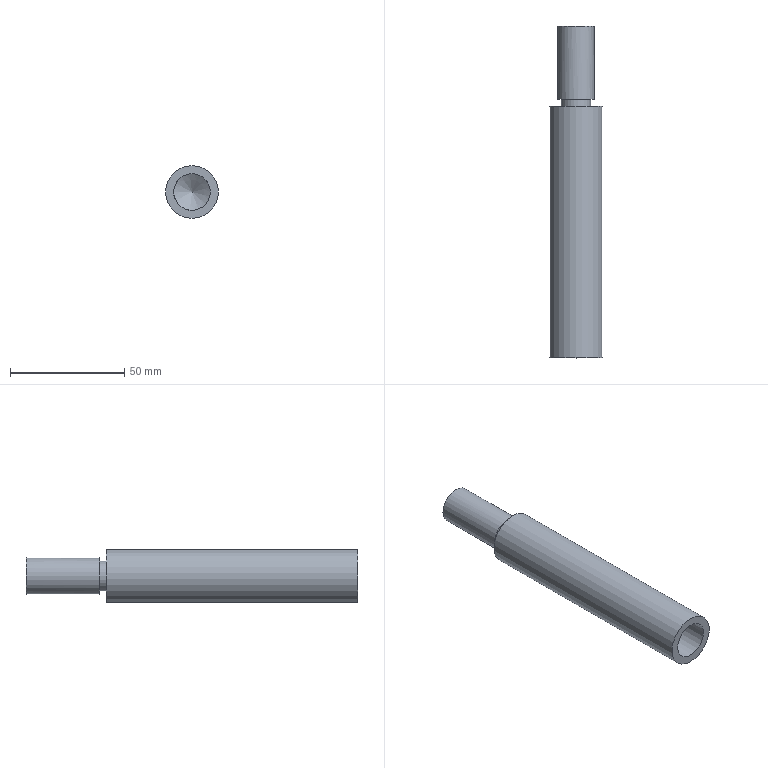Part | NX | features solid 2 | 1 solid | 9 faces | box 23 x 145 x 23 mm | volume 41355 mm3 | cylinder 4 | plane 4 | cone 1 | commonest cylinder face diameters 16 x2 13 x1 23 x1
STEP:
#1=CARTESIAN_POINT('',(288.,604.,-380.));
#2=VERTEX_POINT('',#1);
#3=CARTESIAN_POINT('',(280.,604.,-380.));
#4=DIRECTION('',(0.,-1.,0.));
#5=DIRECTION('',(1.,0.,0.));
#6=AXIS2_PLACEMENT_3D('',#3,#4,#5);
#7=CIRCLE('',#6,8.);
#8=EDGE_CURVE('',#2,#2,#7,.T.);
#9=ORIENTED_EDGE('',*,*,#8,.T.);
#10=EDGE_LOOP('',(#9));
#11=FACE_BOUND('',#10,.T.);
#12=CARTESIAN_POINT('',(280.,608.807,-380.));
#13=VERTEX_POINT('',#12);
#14=VERTEX_LOOP('',#13);
#15=FACE_BOUND('',#14,.T.);
#16=CARTESIAN_POINT('',(280.,604.,-380.));
#17=DIRECTION('',(0.,-1.,0.));
#18=DIRECTION('',(-1.,0.,0.));
#19=AXIS2_PLACEMENT_3D('',#16,#17,#18);
#20=CONICAL_SURFACE('',#19,8.,1.03);
#21=ADVANCED_FACE('',(#11,#15),#20,.F.);
#22=ORIENTED_EDGE('',*,*,#8,.F.);
#23=EDGE_LOOP('',(#22));
#24=FACE_BOUND('',#23,.T.);
#25=CARTESIAN_POINT('',(280.,550.,-372.));
#26=VERTEX_POINT('',#25);
#27=CARTESIAN_POINT('',(280.,550.,-380.));
#28=DIRECTION('',(0.,1.,0.));
#29=DIRECTION('',(0.,0.,1.));
#30=AXIS2_PLACEMENT_3D('',#27,#28,#29);
#31=CIRCLE('',#30,8.);
#32=EDGE_CURVE('',#26,#26,#31,.F.);
#33=ORIENTED_EDGE('',*,*,#32,.T.);
#34=EDGE_LOOP('',(#33));
#35=FACE_BOUND('',#34,.T.);
#36=CARTESIAN_POINT('',(280.,579.,-380.));
#37=DIRECTION('',(0.,1.,0.));
#38=DIRECTION('',(1.,0.,0.));
#39=AXIS2_PLACEMENT_3D('',#36,#37,#38);
#40=CYLINDRICAL_SURFACE('',#39,8.);
#41=ADVANCED_FACE('',(#24,#35),#40,.F.);
#42=CARTESIAN_POINT('',(280.,550.,-368.5));
#43=VERTEX_POINT('',#42);
#44=CARTESIAN_POINT('',(280.,550.,-380.));
#45=DIRECTION('',(0.,1.,0.));
#46=DIRECTION('',(0.,0.,1.));
#47=AXIS2_PLACEMENT_3D('',#44,#45,#46);
#48=CIRCLE('',#47,11.5);
#49=EDGE_CURVE('',#43,#43,#48,.T.);
#50=ORIENTED_EDGE('',*,*,#49,.F.);
#51=EDGE_LOOP('',(#50));
#52=FACE_BOUND('',#51,.T.);
#53=ORIENTED_EDGE('',*,*,#32,.F.);
#54=EDGE_LOOP('',(#53));
#55=FACE_BOUND('',#54,.T.);
#56=CARTESIAN_POINT('',(280.,550.,-380.));
#57=DIRECTION('',(0.,-1.,0.));
#58=DIRECTION('',(-1.,0.,0.));
#59=AXIS2_PLACEMENT_3D('',#56,#57,#58);
#60=PLANE('',#59);
#61=ADVANCED_FACE('',(#52,#55),#60,.T.);
#62=ORIENTED_EDGE('',*,*,#49,.T.);
#63=EDGE_LOOP('',(#62));
#64=FACE_BOUND('',#63,.T.);
#65=CARTESIAN_POINT('',(270.34,650.,-373.76));
#66=VERTEX_POINT('',#65);
#67=CARTESIAN_POINT('',(270.34,635.,-373.76));
#68=VERTEX_POINT('',#67);
#69=CARTESIAN_POINT('',(270.34,508.,-373.76));
#70=DIRECTION('',(0.,1.,0.));
#71=VECTOR('',#70,1000.);
#72=LINE('',#69,#71);
#73=EDGE_CURVE('',#66,#68,#72,.F.);
#74=ORIENTED_EDGE('',*,*,#73,.T.);
#75=ORIENTED_EDGE('',*,*,#73,.F.);
#76=EDGE_LOOP('',(#74,#75));
#77=FACE_BOUND('',#76,.T.);
#78=CARTESIAN_POINT('',(289.66,650.,-386.24));
#79=VERTEX_POINT('',#78);
#80=CARTESIAN_POINT('',(289.66,635.,-386.24));
#81=VERTEX_POINT('',#80);
#82=CARTESIAN_POINT('',(289.66,508.,-386.24));
#83=DIRECTION('',(0.,1.,0.));
#84=VECTOR('',#83,1000.);
#85=LINE('',#82,#84);
#86=EDGE_CURVE('',#79,#81,#85,.F.);
#87=ORIENTED_EDGE('',*,*,#86,.T.);
#88=ORIENTED_EDGE('',*,*,#86,.F.);
#89=EDGE_LOOP('',(#87,#88));
#90=FACE_BOUND('',#89,.T.);
#91=CARTESIAN_POINT('',(280.,660.,-368.5));
#92=VERTEX_POINT('',#91);
#93=CARTESIAN_POINT('',(280.,660.,-380.));
#94=DIRECTION('',(0.,1.,0.));
#95=DIRECTION('',(0.,0.,1.));
#96=AXIS2_PLACEMENT_3D('',#93,#94,#95);
#97=CIRCLE('',#96,11.5);
#98=EDGE_CURVE('',#92,#92,#97,.T.);
#99=ORIENTED_EDGE('',*,*,#98,.F.);
#100=EDGE_LOOP('',(#99));
#101=FACE_BOUND('',#100,.T.);
#102=CARTESIAN_POINT('',(270.34,650.,-386.24));
#103=VERTEX_POINT('',#102);
#104=CARTESIAN_POINT('',(270.34,635.,-386.24));
#105=VERTEX_POINT('',#104);
#106=CARTESIAN_POINT('',(270.34,508.,-386.24));
#107=DIRECTION('',(0.,1.,0.));
#108=VECTOR('',#107,1000.);
#109=LINE('',#106,#108);
#110=EDGE_CURVE('',#103,#105,#109,.F.);
#111=ORIENTED_EDGE('',*,*,#110,.T.);
#112=ORIENTED_EDGE('',*,*,#110,.F.);
#113=EDGE_LOOP('',(#111,#112));
#114=FACE_BOUND('',#113,.T.);
#115=CARTESIAN_POINT('',(289.66,650.,-373.76));
#116=VERTEX_POINT('',#115);
#117=CARTESIAN_POINT('',(289.66,635.,-373.76));
#118=VERTEX_POINT('',#117);
#119=CARTESIAN_POINT('',(289.66,508.,-373.76));
#120=DIRECTION('',(0.,1.,0.));
#121=VECTOR('',#120,1000.);
#122=LINE('',#119,#121);
#123=EDGE_CURVE('',#116,#118,#122,.F.);
#124=ORIENTED_EDGE('',*,*,#123,.T.);
#125=ORIENTED_EDGE('',*,*,#123,.F.);
#126=EDGE_LOOP('',(#124,#125));
#127=FACE_BOUND('',#126,.T.);
#128=CARTESIAN_POINT('',(280.,579.,-380.));
#129=DIRECTION('',(0.,1.,0.));
#130=DIRECTION('',(1.,0.,0.));
#131=AXIS2_PLACEMENT_3D('',#128,#129,#130);
#132=CYLINDRICAL_SURFACE('',#131,11.5);
#133=ADVANCED_FACE('',(#64,#77,#90,#101,#114,#127),#132,.T.);
#134=CARTESIAN_POINT('',(272.,663.,-380.));
#135=VERTEX_POINT('',#134);
#136=CARTESIAN_POINT('',(280.,663.,-380.));
#137=DIRECTION('',(0.,1.,0.));
#138=DIRECTION('',(-1.,0.,0.));
#139=AXIS2_PLACEMENT_3D('',#136,#137,#138);
#140=CIRCLE('',#139,8.);
#141=EDGE_CURVE('',#135,#135,#140,.T.);
#142=ORIENTED_EDGE('',*,*,#141,.T.);
#143=EDGE_LOOP('',(#142));
#144=FACE_BOUND('',#143,.T.);
#145=CARTESIAN_POINT('',(280.,695.,-372.));
#146=VERTEX_POINT('',#145);
#147=CARTESIAN_POINT('',(280.,695.,-380.));
#148=DIRECTION('',(0.,1.,0.));
#149=DIRECTION('',(0.,0.,1.));
#150=AXIS2_PLACEMENT_3D('',#147,#148,#149);
#151=CIRCLE('',#150,8.);
#152=EDGE_CURVE('',#146,#146,#151,.T.);
#153=ORIENTED_EDGE('',*,*,#152,.F.);
#154=EDGE_LOOP('',(#153));
#155=FACE_BOUND('',#154,.T.);
#156=CARTESIAN_POINT('',(280.,677.,-380.));
#157=DIRECTION('',(0.,-1.,0.));
#158=DIRECTION('',(-1.,0.,0.));
#159=AXIS2_PLACEMENT_3D('',#156,#157,#158);
#160=CYLINDRICAL_SURFACE('',#159,8.);
#161=ADVANCED_FACE('',(#144,#155),#160,.T.);
#162=CARTESIAN_POINT('',(273.5,663.,-380.));
#163=VERTEX_POINT('',#162);
#164=CARTESIAN_POINT('',(280.,663.,-380.));
#165=DIRECTION('',(0.,1.,0.));
#166=DIRECTION('',(-1.,0.,0.));
#167=AXIS2_PLACEMENT_3D('',#164,#165,#166);
#168=CIRCLE('',#167,6.5);
#169=EDGE_CURVE('',#163,#163,#168,.F.);
#170=ORIENTED_EDGE('',*,*,#169,.T.);
#171=EDGE_LOOP('',(#170));
#172=FACE_BOUND('',#171,.T.);
#173=CARTESIAN_POINT('',(273.5,660.,-380.));
#174=VERTEX_POINT('',#173);
#175=CARTESIAN_POINT('',(280.,660.,-380.));
#176=DIRECTION('',(0.,1.,0.));
#177=DIRECTION('',(-1.,0.,0.));
#178=AXIS2_PLACEMENT_3D('',#175,#176,#177);
#179=CIRCLE('',#178,6.5);
#180=EDGE_CURVE('',#174,#174,#179,.T.);
#181=ORIENTED_EDGE('',*,*,#180,.T.);
#182=EDGE_LOOP('',(#181));
#183=FACE_BOUND('',#182,.T.);
#184=CARTESIAN_POINT('',(280.,663.,-380.));
#185=DIRECTION('',(0.,-1.,0.));
#186=DIRECTION('',(-1.,0.,0.));
#187=AXIS2_PLACEMENT_3D('',#184,#185,#186);
#188=CYLINDRICAL_SURFACE('',#187,6.5);
#189=ADVANCED_FACE('',(#172,#183),#188,.T.);
#190=ORIENTED_EDGE('',*,*,#152,.T.);
#191=EDGE_LOOP('',(#190));
#192=FACE_BOUND('',#191,.T.);
#193=CARTESIAN_POINT('',(250.,695.,-410.));
#194=DIRECTION('',(0.,-1.,0.));
#195=DIRECTION('',(-1.,0.,0.));
#196=AXIS2_PLACEMENT_3D('',#193,#194,#195);
#197=PLANE('',#196);
#198=ADVANCED_FACE('',(#192),#197,.F.);
#199=ORIENTED_EDGE('',*,*,#169,.F.);
#200=EDGE_LOOP('',(#199));
#201=FACE_BOUND('',#200,.T.);
#202=ORIENTED_EDGE('',*,*,#141,.F.);
#203=EDGE_LOOP('',(#202));
#204=FACE_BOUND('',#203,.T.);
#205=CARTESIAN_POINT('',(280.,663.,-380.));
#206=DIRECTION('',(0.,-1.,0.));
#207=DIRECTION('',(-1.,0.,0.));
#208=AXIS2_PLACEMENT_3D('',#205,#206,#207);
#209=PLANE('',#208);
#210=ADVANCED_FACE('',(#201,#204),#209,.T.);
#211=ORIENTED_EDGE('',*,*,#180,.F.);
#212=EDGE_LOOP('',(#211));
#213=FACE_BOUND('',#212,.T.);
#214=ORIENTED_EDGE('',*,*,#98,.T.);
#215=EDGE_LOOP('',(#214));
#216=FACE_BOUND('',#215,.T.);
#217=CARTESIAN_POINT('',(280.,660.,-380.));
#218=DIRECTION('',(0.,-1.,0.));
#219=DIRECTION('',(-1.,0.,0.));
#220=AXIS2_PLACEMENT_3D('',#217,#218,#219);
#221=PLANE('',#220);
#222=ADVANCED_FACE('',(#213,#216),#221,.F.);
#223=CLOSED_SHELL('',(#21,#41,#61,#133,#161,#189,#198,#210,#222));
#224=MANIFOLD_SOLID_BREP('',#223);
#225=(LENGTH_UNIT()NAMED_UNIT(*)SI_UNIT(.MILLI.,.METRE.));
#226=UNCERTAINTY_MEASURE_WITH_UNIT(LENGTH_MEASURE(0.00001),#225,'','');
#227=(NAMED_UNIT(*)PLANE_ANGLE_UNIT()SI_UNIT($,.RADIAN.));
#228=(NAMED_UNIT(*)SI_UNIT($,.STERADIAN.)SOLID_ANGLE_UNIT());
#229=(GEOMETRIC_REPRESENTATION_CONTEXT(3)GLOBAL_UNCERTAINTY_ASSIGNED_CONTEXT((#226))GLOBAL_UNIT_ASSIGNED_CONTEXT((#225,#227,#228))REPRESENTATION_CONTEXT('',''));
#230=ADVANCED_BREP_SHAPE_REPRESENTATION('',(#224),#229);